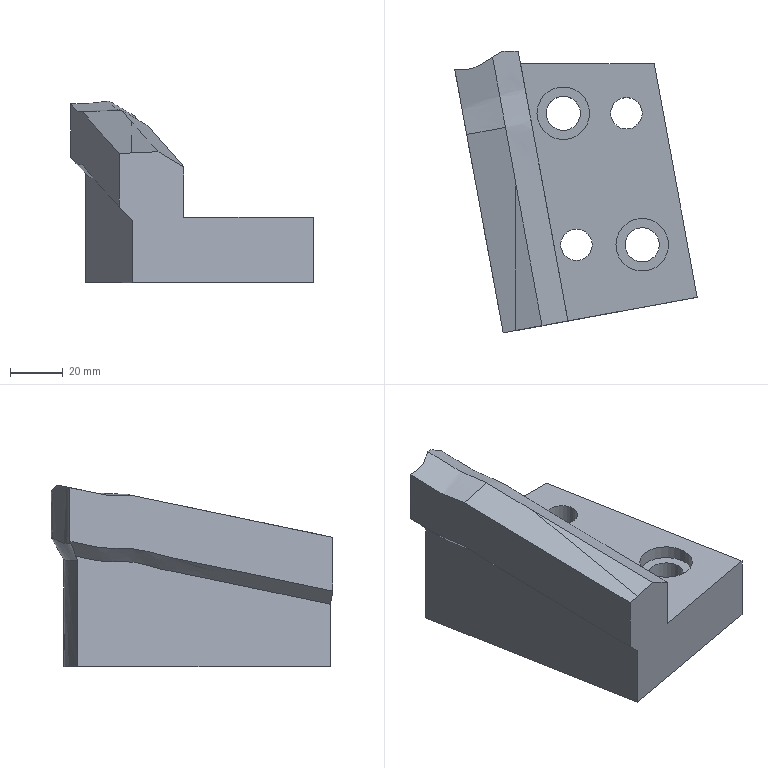Part | NX | features solid 2 | 1 solid | 23 faces | box 92.15 x 107.047 x 69.178 mm | volume 233289 mm3 | plane 9 | spline 8 | cylinder 6 | commonest cylinder face diameters 12 x2 13 x2 20 x2